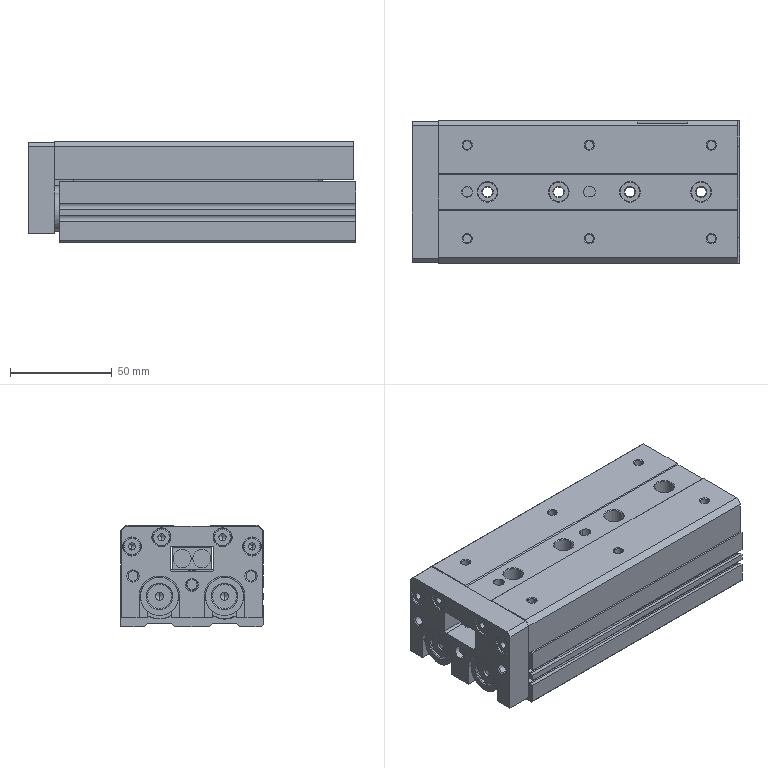Part | STEP file | 2 solids | 483 faces | box 161 x 70 x 50 mm | volume 433153 mm3 | cylinder 192 | plane 163 | cone 118 | torus 10 | commonest cylinder face diameters 4.134 x24 4.917 x20 9 x16 9.5 x14 10 x12 20 x12